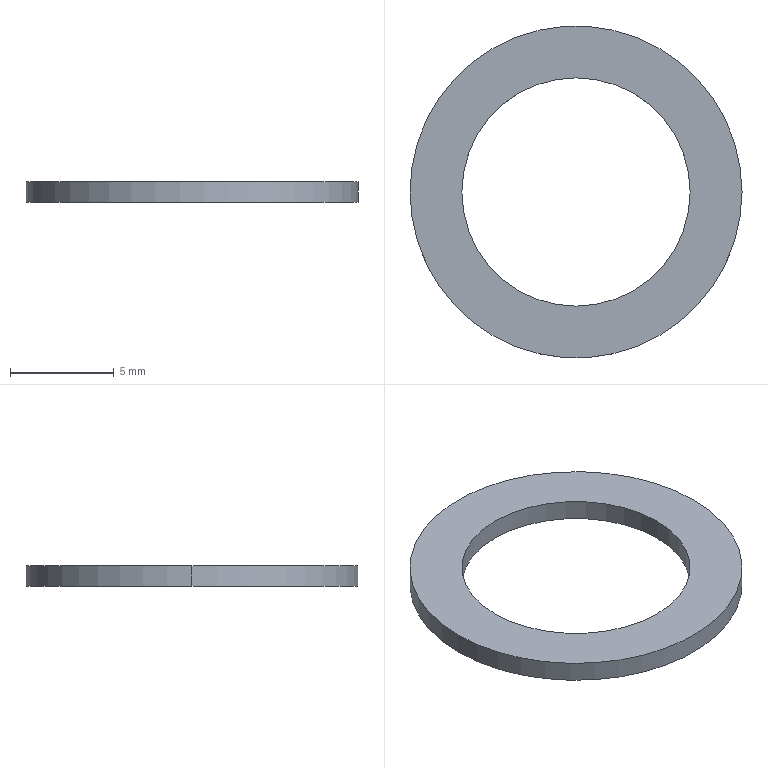Part | SolidWorks | features Extrusion 1 | 1 solid | 6 faces | box 16 x 16 x 1 mm | volume 106.029 mm3 | cylinder 4 | plane 2 | commonest cylinder face diameters 11 x2 16 x2
STEP:
#1=CARTESIAN_POINT('',(-5.5,0.,1.));
#2=VERTEX_POINT('',#1);
#3=CARTESIAN_POINT('',(5.5,0.,1.));
#4=VERTEX_POINT('',#3);
#5=CARTESIAN_POINT('',(0.,0.,1.));
#6=DIRECTION('',(0.,0.,1.));
#7=DIRECTION('',(1.,0.,0.));
#8=AXIS2_PLACEMENT_3D('',#5,#6,#7);
#9=CIRCLE('',#8,5.5);
#10=EDGE_CURVE('',#2,#4,#9,.T.);
#11=ORIENTED_EDGE('',*,*,#10,.T.);
#12=CARTESIAN_POINT('',(5.5,0.,0.));
#13=VERTEX_POINT('',#12);
#14=CARTESIAN_POINT('',(5.5,0.,1.));
#15=DIRECTION('',(0.,0.,-1.));
#16=VECTOR('',#15,1000.);
#17=LINE('',#14,#16);
#18=EDGE_CURVE('',#4,#13,#17,.T.);
#19=ORIENTED_EDGE('',*,*,#18,.T.);
#20=CARTESIAN_POINT('',(-5.5,0.,0.));
#21=VERTEX_POINT('',#20);
#22=CARTESIAN_POINT('',(0.,0.,0.));
#23=DIRECTION('',(0.,0.,1.));
#24=DIRECTION('',(1.,0.,0.));
#25=AXIS2_PLACEMENT_3D('',#22,#23,#24);
#26=CIRCLE('',#25,5.5);
#27=EDGE_CURVE('',#21,#13,#26,.T.);
#28=ORIENTED_EDGE('',*,*,#27,.F.);
#29=CARTESIAN_POINT('',(-5.5,0.,1.));
#30=DIRECTION('',(0.,0.,-1.));
#31=VECTOR('',#30,1000.);
#32=LINE('',#29,#31);
#33=EDGE_CURVE('',#2,#21,#32,.T.);
#34=ORIENTED_EDGE('',*,*,#33,.F.);
#35=EDGE_LOOP('',(#11,#19,#28,#34));
#36=FACE_OUTER_BOUND('',#35,.T.);
#37=CARTESIAN_POINT('',(0.,0.,1.));
#38=DIRECTION('',(0.,0.,-1.));
#39=DIRECTION('',(-1.,0.,0.));
#40=AXIS2_PLACEMENT_3D('',#37,#38,#39);
#41=CYLINDRICAL_SURFACE('',#40,5.5);
#42=ADVANCED_FACE('',(#36),#41,.F.);
#43=CARTESIAN_POINT('',(8.,0.,1.));
#44=VERTEX_POINT('',#43);
#45=CARTESIAN_POINT('',(-8.,0.,1.));
#46=VERTEX_POINT('',#45);
#47=CARTESIAN_POINT('',(0.,0.,1.));
#48=DIRECTION('',(0.,0.,1.));
#49=DIRECTION('',(1.,0.,0.));
#50=AXIS2_PLACEMENT_3D('',#47,#48,#49);
#51=CIRCLE('',#50,8.);
#52=EDGE_CURVE('',#44,#46,#51,.T.);
#53=ORIENTED_EDGE('',*,*,#52,.F.);
#54=CARTESIAN_POINT('',(8.,0.,0.));
#55=VERTEX_POINT('',#54);
#56=CARTESIAN_POINT('',(8.,0.,1.));
#57=DIRECTION('',(0.,0.,-1.));
#58=VECTOR('',#57,1000.);
#59=LINE('',#56,#58);
#60=EDGE_CURVE('',#44,#55,#59,.T.);
#61=ORIENTED_EDGE('',*,*,#60,.T.);
#62=CARTESIAN_POINT('',(-8.,0.,0.));
#63=VERTEX_POINT('',#62);
#64=CARTESIAN_POINT('',(0.,0.,0.));
#65=DIRECTION('',(0.,0.,1.));
#66=DIRECTION('',(1.,0.,0.));
#67=AXIS2_PLACEMENT_3D('',#64,#65,#66);
#68=CIRCLE('',#67,8.);
#69=EDGE_CURVE('',#55,#63,#68,.T.);
#70=ORIENTED_EDGE('',*,*,#69,.T.);
#71=CARTESIAN_POINT('',(-8.,0.,1.));
#72=DIRECTION('',(0.,0.,-1.));
#73=VECTOR('',#72,1000.);
#74=LINE('',#71,#73);
#75=EDGE_CURVE('',#46,#63,#74,.T.);
#76=ORIENTED_EDGE('',*,*,#75,.F.);
#77=EDGE_LOOP('',(#53,#61,#70,#76));
#78=FACE_OUTER_BOUND('',#77,.T.);
#79=CARTESIAN_POINT('',(0.,0.,1.));
#80=DIRECTION('',(0.,0.,-1.));
#81=DIRECTION('',(-1.,0.,0.));
#82=AXIS2_PLACEMENT_3D('',#79,#80,#81);
#83=CYLINDRICAL_SURFACE('',#82,8.);
#84=ADVANCED_FACE('',(#78),#83,.T.);
#85=CARTESIAN_POINT('',(0.,0.,1.));
#86=DIRECTION('',(0.,0.,1.));
#87=DIRECTION('',(1.,0.,0.));
#88=AXIS2_PLACEMENT_3D('',#85,#86,#87);
#89=CIRCLE('',#88,8.);
#90=EDGE_CURVE('',#46,#44,#89,.T.);
#91=ORIENTED_EDGE('',*,*,#90,.T.);
#92=ORIENTED_EDGE('',*,*,#52,.T.);
#93=EDGE_LOOP('',(#91,#92));
#94=FACE_OUTER_BOUND('',#93,.T.);
#95=ORIENTED_EDGE('',*,*,#10,.F.);
#96=CARTESIAN_POINT('',(0.,0.,1.));
#97=DIRECTION('',(0.,0.,1.));
#98=DIRECTION('',(1.,0.,0.));
#99=AXIS2_PLACEMENT_3D('',#96,#97,#98);
#100=CIRCLE('',#99,5.5);
#101=EDGE_CURVE('',#4,#2,#100,.T.);
#102=ORIENTED_EDGE('',*,*,#101,.F.);
#103=EDGE_LOOP('',(#95,#102));
#104=FACE_BOUND('',#103,.T.);
#105=CARTESIAN_POINT('',(0.,0.,1.));
#106=DIRECTION('',(0.,0.,1.));
#107=DIRECTION('',(1.,0.,0.));
#108=AXIS2_PLACEMENT_3D('',#105,#106,#107);
#109=PLANE('',#108);
#110=ADVANCED_FACE('',(#94,#104),#109,.T.);
#111=CARTESIAN_POINT('',(0.,0.,0.));
#112=DIRECTION('',(0.,0.,1.));
#113=DIRECTION('',(1.,0.,0.));
#114=AXIS2_PLACEMENT_3D('',#111,#112,#113);
#115=CIRCLE('',#114,8.);
#116=EDGE_CURVE('',#63,#55,#115,.T.);
#117=ORIENTED_EDGE('',*,*,#116,.F.);
#118=ORIENTED_EDGE('',*,*,#69,.F.);
#119=EDGE_LOOP('',(#117,#118));
#120=FACE_OUTER_BOUND('',#119,.T.);
#121=ORIENTED_EDGE('',*,*,#27,.T.);
#122=CARTESIAN_POINT('',(0.,0.,0.));
#123=DIRECTION('',(0.,0.,1.));
#124=DIRECTION('',(1.,0.,0.));
#125=AXIS2_PLACEMENT_3D('',#122,#123,#124);
#126=CIRCLE('',#125,5.5);
#127=EDGE_CURVE('',#13,#21,#126,.T.);
#128=ORIENTED_EDGE('',*,*,#127,.T.);
#129=EDGE_LOOP('',(#121,#128));
#130=FACE_BOUND('',#129,.T.);
#131=CARTESIAN_POINT('',(0.,0.,0.));
#132=DIRECTION('',(0.,0.,1.));
#133=DIRECTION('',(1.,0.,0.));
#134=AXIS2_PLACEMENT_3D('',#131,#132,#133);
#135=PLANE('',#134);
#136=ADVANCED_FACE('',(#120,#130),#135,.F.);
#137=ORIENTED_EDGE('',*,*,#60,.F.);
#138=ORIENTED_EDGE('',*,*,#90,.F.);
#139=ORIENTED_EDGE('',*,*,#75,.T.);
#140=ORIENTED_EDGE('',*,*,#116,.T.);
#141=EDGE_LOOP('',(#137,#138,#139,#140));
#142=FACE_OUTER_BOUND('',#141,.T.);
#143=CARTESIAN_POINT('',(0.,0.,1.));
#144=DIRECTION('',(0.,0.,-1.));
#145=DIRECTION('',(-1.,0.,0.));
#146=AXIS2_PLACEMENT_3D('',#143,#144,#145);
#147=CYLINDRICAL_SURFACE('',#146,8.);
#148=ADVANCED_FACE('',(#142),#147,.T.);
#149=ORIENTED_EDGE('',*,*,#18,.F.);
#150=ORIENTED_EDGE('',*,*,#101,.T.);
#151=ORIENTED_EDGE('',*,*,#33,.T.);
#152=ORIENTED_EDGE('',*,*,#127,.F.);
#153=EDGE_LOOP('',(#149,#150,#151,#152));
#154=FACE_OUTER_BOUND('',#153,.T.);
#155=CARTESIAN_POINT('',(0.,0.,1.));
#156=DIRECTION('',(0.,0.,-1.));
#157=DIRECTION('',(-1.,0.,0.));
#158=AXIS2_PLACEMENT_3D('',#155,#156,#157);
#159=CYLINDRICAL_SURFACE('',#158,5.5);
#160=ADVANCED_FACE('',(#154),#159,.F.);
#161=CLOSED_SHELL('',(#42,#84,#110,#136,#148,#160));
#162=MANIFOLD_SOLID_BREP('',#161);
#163=CARTESIAN_POINT('',(0.,0.,0.));
#164=DIRECTION('',(0.,0.,1.));
#165=DIRECTION('',(1.,0.,0.));
#166=AXIS2_PLACEMENT_3D('',#163,#164,#165);
#167=(LENGTH_UNIT()NAMED_UNIT(*)SI_UNIT(.MILLI.,.METRE.));
#168=UNCERTAINTY_MEASURE_WITH_UNIT(LENGTH_MEASURE(0.00001),#167,'','');
#169=(NAMED_UNIT(*)PLANE_ANGLE_UNIT()SI_UNIT($,.RADIAN.));
#170=(NAMED_UNIT(*)SI_UNIT($,.STERADIAN.)SOLID_ANGLE_UNIT());
#171=(GEOMETRIC_REPRESENTATION_CONTEXT(3)GLOBAL_UNCERTAINTY_ASSIGNED_CONTEXT((#168))GLOBAL_UNIT_ASSIGNED_CONTEXT((#167,#169,#170))REPRESENTATION_CONTEXT('',''));
#172=ADVANCED_BREP_SHAPE_REPRESENTATION('',(#162,#166),#171);